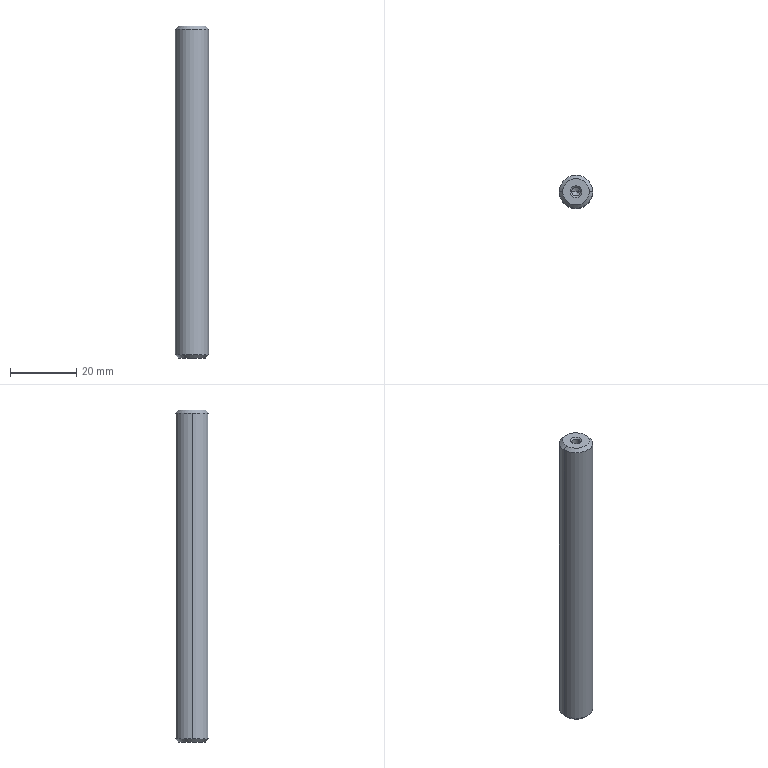Part | SolidWorks | features Chamfer 2, Extrusion 1, HoleWzd 1 | 1 solid | 14 faces | box 10 x 10 x 100 mm | volume 7790 mm3 | cone 8 | cylinder 4 | plane 2 | commonest cylinder face diameters 2.5 x2 10 x2
STEP:
#1=CARTESIAN_POINT('',(-1.25,0.,99.5));
#2=VERTEX_POINT('',#1);
#3=CARTESIAN_POINT('',(1.25,0.,99.5));
#4=VERTEX_POINT('',#3);
#5=CARTESIAN_POINT('',(0.,0.,99.5));
#6=DIRECTION('',(0.,0.,1.));
#7=DIRECTION('',(1.,0.,0.));
#8=AXIS2_PLACEMENT_3D('',#5,#6,#7);
#9=CIRCLE('',#8,1.25);
#10=EDGE_CURVE('',#2,#4,#9,.T.);
#11=ORIENTED_EDGE('',*,*,#10,.F.);
#12=CARTESIAN_POINT('',(-1.75,0.,100.));
#13=VERTEX_POINT('',#12);
#14=CARTESIAN_POINT('',(-1.25,0.,99.5));
#15=DIRECTION('',(-0.7071,0.,0.7071));
#16=VECTOR('',#15,1000.);
#17=LINE('',#14,#16);
#18=EDGE_CURVE('',#2,#13,#17,.T.);
#19=ORIENTED_EDGE('',*,*,#18,.T.);
#20=CARTESIAN_POINT('',(1.75,0.,100.));
#21=VERTEX_POINT('',#20);
#22=CARTESIAN_POINT('',(0.,0.,100.));
#23=DIRECTION('',(0.,0.,-1.));
#24=DIRECTION('',(1.,0.,0.));
#25=AXIS2_PLACEMENT_3D('',#22,#23,#24);
#26=CIRCLE('',#25,1.75);
#27=EDGE_CURVE('',#21,#13,#26,.T.);
#28=ORIENTED_EDGE('',*,*,#27,.F.);
#29=CARTESIAN_POINT('',(1.25,0.,99.5));
#30=DIRECTION('',(0.7071,0.,0.7071));
#31=VECTOR('',#30,1000.);
#32=LINE('',#29,#31);
#33=EDGE_CURVE('',#4,#21,#32,.T.);
#34=ORIENTED_EDGE('',*,*,#33,.F.);
#35=EDGE_LOOP('',(#11,#19,#28,#34));
#36=FACE_OUTER_BOUND('',#35,.T.);
#37=CARTESIAN_POINT('',(0.,0.,99.5));
#38=DIRECTION('',(0.,0.,1.));
#39=DIRECTION('',(1.,0.,0.));
#40=AXIS2_PLACEMENT_3D('',#37,#38,#39);
#41=CONICAL_SURFACE('',#40,1.25,0.7854);
#42=ADVANCED_FACE('',(#36),#41,.F.);
#43=CARTESIAN_POINT('',(4.,0.,100.));
#44=VERTEX_POINT('',#43);
#45=CARTESIAN_POINT('',(-4.,0.,100.));
#46=VERTEX_POINT('',#45);
#47=CARTESIAN_POINT('',(0.,0.,100.));
#48=DIRECTION('',(0.,0.,1.));
#49=DIRECTION('',(1.,0.,0.));
#50=AXIS2_PLACEMENT_3D('',#47,#48,#49);
#51=CIRCLE('',#50,4.);
#52=EDGE_CURVE('',#44,#46,#51,.T.);
#53=ORIENTED_EDGE('',*,*,#52,.F.);
#54=CARTESIAN_POINT('',(5.,0.,99.));
#55=VERTEX_POINT('',#54);
#56=CARTESIAN_POINT('',(4.,0.,100.));
#57=DIRECTION('',(0.7071,0.,-0.7071));
#58=VECTOR('',#57,1000.);
#59=LINE('',#56,#58);
#60=EDGE_CURVE('',#44,#55,#59,.T.);
#61=ORIENTED_EDGE('',*,*,#60,.T.);
#62=CARTESIAN_POINT('',(-5.,0.,99.));
#63=VERTEX_POINT('',#62);
#64=CARTESIAN_POINT('',(0.,0.,99.));
#65=DIRECTION('',(0.,0.,-1.));
#66=DIRECTION('',(1.,0.,0.));
#67=AXIS2_PLACEMENT_3D('',#64,#65,#66);
#68=CIRCLE('',#67,5.);
#69=EDGE_CURVE('',#63,#55,#68,.T.);
#70=ORIENTED_EDGE('',*,*,#69,.F.);
#71=CARTESIAN_POINT('',(-4.,0.,100.));
#72=DIRECTION('',(-0.7071,0.,-0.7071));
#73=VECTOR('',#72,1000.);
#74=LINE('',#71,#73);
#75=EDGE_CURVE('',#46,#63,#74,.T.);
#76=ORIENTED_EDGE('',*,*,#75,.F.);
#77=EDGE_LOOP('',(#53,#61,#70,#76));
#78=FACE_OUTER_BOUND('',#77,.T.);
#79=CARTESIAN_POINT('',(0.,0.,100.));
#80=DIRECTION('',(0.,0.,-1.));
#81=DIRECTION('',(-1.,0.,0.));
#82=AXIS2_PLACEMENT_3D('',#79,#80,#81);
#83=CONICAL_SURFACE('',#82,4.,0.7854);
#84=ADVANCED_FACE('',(#78),#83,.T.);
#85=CARTESIAN_POINT('',(-4.,0.,0.));
#86=VERTEX_POINT('',#85);
#87=CARTESIAN_POINT('',(4.,0.,0.));
#88=VERTEX_POINT('',#87);
#89=CARTESIAN_POINT('',(0.,0.,0.));
#90=DIRECTION('',(0.,0.,-1.));
#91=DIRECTION('',(1.,0.,0.));
#92=AXIS2_PLACEMENT_3D('',#89,#90,#91);
#93=CIRCLE('',#92,4.);
#94=EDGE_CURVE('',#86,#88,#93,.T.);
#95=ORIENTED_EDGE('',*,*,#94,.F.);
#96=CARTESIAN_POINT('',(-5.,0.,1.));
#97=VERTEX_POINT('',#96);
#98=CARTESIAN_POINT('',(-5.,0.,1.));
#99=DIRECTION('',(-0.7071,0.,0.7071));
#100=VECTOR('',#99,1000.);
#101=LINE('',#98,#100);
#102=EDGE_CURVE('',#86,#97,#101,.T.);
#103=ORIENTED_EDGE('',*,*,#102,.T.);
#104=CARTESIAN_POINT('',(5.,0.,1.));
#105=VERTEX_POINT('',#104);
#106=CARTESIAN_POINT('',(0.,0.,1.));
#107=DIRECTION('',(0.,0.,1.));
#108=DIRECTION('',(1.,0.,0.));
#109=AXIS2_PLACEMENT_3D('',#106,#107,#108);
#110=CIRCLE('',#109,5.);
#111=EDGE_CURVE('',#105,#97,#110,.T.);
#112=ORIENTED_EDGE('',*,*,#111,.F.);
#113=CARTESIAN_POINT('',(5.,0.,1.));
#114=DIRECTION('',(0.7071,0.,0.7071));
#115=VECTOR('',#114,1000.);
#116=LINE('',#113,#115);
#117=EDGE_CURVE('',#88,#105,#116,.T.);
#118=ORIENTED_EDGE('',*,*,#117,.F.);
#119=EDGE_LOOP('',(#95,#103,#112,#118));
#120=FACE_OUTER_BOUND('',#119,.T.);
#121=CARTESIAN_POINT('',(0.,0.,1.));
#122=DIRECTION('',(0.,0.,1.));
#123=DIRECTION('',(1.,0.,0.));
#124=AXIS2_PLACEMENT_3D('',#121,#122,#123);
#125=CONICAL_SURFACE('',#124,5.,0.7854);
#126=ADVANCED_FACE('',(#120),#125,.T.);
#127=CARTESIAN_POINT('',(-1.25,0.,93.5));
#128=VERTEX_POINT('',#127);
#129=CARTESIAN_POINT('',(1.25,0.,93.5));
#130=VERTEX_POINT('',#129);
#131=CARTESIAN_POINT('',(0.,0.,93.5));
#132=DIRECTION('',(0.,0.,1.));
#133=DIRECTION('',(1.,0.,0.));
#134=AXIS2_PLACEMENT_3D('',#131,#132,#133);
#135=CIRCLE('',#134,1.25);
#136=EDGE_CURVE('',#128,#130,#135,.T.);
#137=ORIENTED_EDGE('',*,*,#136,.F.);
#138=CARTESIAN_POINT('',(-1.25,0.,100.));
#139=DIRECTION('',(0.,0.,1.));
#140=VECTOR('',#139,1000.);
#141=LINE('',#138,#140);
#142=EDGE_CURVE('',#128,#2,#141,.T.);
#143=ORIENTED_EDGE('',*,*,#142,.T.);
#144=ORIENTED_EDGE('',*,*,#10,.T.);
#145=CARTESIAN_POINT('',(1.25,0.,100.));
#146=DIRECTION('',(0.,0.,1.));
#147=VECTOR('',#146,1000.);
#148=LINE('',#145,#147);
#149=EDGE_CURVE('',#130,#4,#148,.T.);
#150=ORIENTED_EDGE('',*,*,#149,.F.);
#151=EDGE_LOOP('',(#137,#143,#144,#150));
#152=FACE_OUTER_BOUND('',#151,.T.);
#153=CARTESIAN_POINT('',(0.,0.,100.));
#154=DIRECTION('',(0.,0.,1.));
#155=DIRECTION('',(1.,0.,0.));
#156=AXIS2_PLACEMENT_3D('',#153,#154,#155);
#157=CYLINDRICAL_SURFACE('',#156,1.25);
#158=ADVANCED_FACE('',(#152),#157,.F.);
#159=CARTESIAN_POINT('',(0.,0.,92.749));
#160=VERTEX_POINT('',#159);
#161=CARTESIAN_POINT('',(1.25,0.,93.5));
#162=DIRECTION('',(0.8572,0.,0.515));
#163=VECTOR('',#162,1000.);
#164=LINE('',#161,#163);
#165=EDGE_CURVE('',#160,#130,#164,.T.);
#166=ORIENTED_EDGE('',*,*,#165,.F.);
#167=CARTESIAN_POINT('',(-1.25,0.,93.5));
#168=DIRECTION('',(-0.8572,0.,0.515));
#169=VECTOR('',#168,1000.);
#170=LINE('',#167,#169);
#171=EDGE_CURVE('',#160,#128,#170,.T.);
#172=ORIENTED_EDGE('',*,*,#171,.T.);
#173=ORIENTED_EDGE('',*,*,#136,.T.);
#174=EDGE_LOOP('',(#166,#172,#173));
#175=FACE_OUTER_BOUND('',#174,.T.);
#176=CARTESIAN_POINT('',(0.,0.,93.5));
#177=DIRECTION('',(0.,0.,1.));
#178=DIRECTION('',(1.,0.,0.));
#179=AXIS2_PLACEMENT_3D('',#176,#177,#178);
#180=CONICAL_SURFACE('',#179,1.25,1.03);
#181=ADVANCED_FACE('',(#175),#180,.F.);
#182=ORIENTED_EDGE('',*,*,#69,.T.);
#183=CARTESIAN_POINT('',(5.,0.,100.));
#184=DIRECTION('',(0.,0.,-1.));
#185=VECTOR('',#184,1000.);
#186=LINE('',#183,#185);
#187=EDGE_CURVE('',#55,#105,#186,.T.);
#188=ORIENTED_EDGE('',*,*,#187,.T.);
#189=ORIENTED_EDGE('',*,*,#111,.T.);
#190=CARTESIAN_POINT('',(-5.,0.,100.));
#191=DIRECTION('',(0.,0.,-1.));
#192=VECTOR('',#191,1000.);
#193=LINE('',#190,#192);
#194=EDGE_CURVE('',#63,#97,#193,.T.);
#195=ORIENTED_EDGE('',*,*,#194,.F.);
#196=EDGE_LOOP('',(#182,#188,#189,#195));
#197=FACE_OUTER_BOUND('',#196,.T.);
#198=CARTESIAN_POINT('',(0.,0.,100.));
#199=DIRECTION('',(0.,0.,-1.));
#200=DIRECTION('',(-1.,0.,0.));
#201=AXIS2_PLACEMENT_3D('',#198,#199,#200);
#202=CYLINDRICAL_SURFACE('',#201,5.);
#203=ADVANCED_FACE('',(#197),#202,.T.);
#204=ORIENTED_EDGE('',*,*,#187,.F.);
#205=CARTESIAN_POINT('',(0.,0.,99.));
#206=DIRECTION('',(0.,0.,-1.));
#207=DIRECTION('',(1.,0.,0.));
#208=AXIS2_PLACEMENT_3D('',#205,#206,#207);
#209=CIRCLE('',#208,5.);
#210=EDGE_CURVE('',#55,#63,#209,.T.);
#211=ORIENTED_EDGE('',*,*,#210,.T.);
#212=ORIENTED_EDGE('',*,*,#194,.T.);
#213=CARTESIAN_POINT('',(0.,0.,1.));
#214=DIRECTION('',(0.,0.,1.));
#215=DIRECTION('',(1.,0.,0.));
#216=AXIS2_PLACEMENT_3D('',#213,#214,#215);
#217=CIRCLE('',#216,5.);
#218=EDGE_CURVE('',#97,#105,#217,.T.);
#219=ORIENTED_EDGE('',*,*,#218,.T.);
#220=EDGE_LOOP('',(#204,#211,#212,#219));
#221=FACE_OUTER_BOUND('',#220,.T.);
#222=CARTESIAN_POINT('',(0.,0.,100.));
#223=DIRECTION('',(0.,0.,-1.));
#224=DIRECTION('',(-1.,0.,0.));
#225=AXIS2_PLACEMENT_3D('',#222,#223,#224);
#226=CYLINDRICAL_SURFACE('',#225,5.);
#227=ADVANCED_FACE('',(#221),#226,.T.);
#228=ORIENTED_EDGE('',*,*,#27,.T.);
#229=CARTESIAN_POINT('',(0.,0.,100.));
#230=DIRECTION('',(0.,0.,-1.));
#231=DIRECTION('',(1.,0.,0.));
#232=AXIS2_PLACEMENT_3D('',#229,#230,#231);
#233=CIRCLE('',#232,1.75);
#234=EDGE_CURVE('',#13,#21,#233,.T.);
#235=ORIENTED_EDGE('',*,*,#234,.T.);
#236=EDGE_LOOP('',(#228,#235));
#237=FACE_BOUND('',#236,.T.);
#238=CARTESIAN_POINT('',(0.,0.,100.));
#239=DIRECTION('',(0.,0.,1.));
#240=DIRECTION('',(1.,0.,0.));
#241=AXIS2_PLACEMENT_3D('',#238,#239,#240);
#242=CIRCLE('',#241,4.);
#243=EDGE_CURVE('',#46,#44,#242,.T.);
#244=ORIENTED_EDGE('',*,*,#243,.T.);
#245=ORIENTED_EDGE('',*,*,#52,.T.);
#246=EDGE_LOOP('',(#244,#245));
#247=FACE_OUTER_BOUND('',#246,.T.);
#248=CARTESIAN_POINT('',(0.,0.,100.));
#249=DIRECTION('',(0.,0.,1.));
#250=DIRECTION('',(1.,0.,0.));
#251=AXIS2_PLACEMENT_3D('',#248,#249,#250);
#252=PLANE('',#251);
#253=ADVANCED_FACE('',(#237,#247),#252,.T.);
#254=CARTESIAN_POINT('',(0.,0.,0.));
#255=DIRECTION('',(0.,0.,-1.));
#256=DIRECTION('',(1.,0.,0.));
#257=AXIS2_PLACEMENT_3D('',#254,#255,#256);
#258=CIRCLE('',#257,4.);
#259=EDGE_CURVE('',#88,#86,#258,.T.);
#260=ORIENTED_EDGE('',*,*,#259,.T.);
#261=ORIENTED_EDGE('',*,*,#94,.T.);
#262=EDGE_LOOP('',(#260,#261));
#263=FACE_OUTER_BOUND('',#262,.T.);
#264=CARTESIAN_POINT('',(0.,0.,0.));
#265=DIRECTION('',(0.,0.,1.));
#266=DIRECTION('',(1.,0.,0.));
#267=AXIS2_PLACEMENT_3D('',#264,#265,#266);
#268=PLANE('',#267);
#269=ADVANCED_FACE('',(#263),#268,.F.);
#270=ORIENTED_EDGE('',*,*,#171,.F.);
#271=ORIENTED_EDGE('',*,*,#165,.T.);
#272=CARTESIAN_POINT('',(0.,0.,93.5));
#273=DIRECTION('',(0.,0.,1.));
#274=DIRECTION('',(1.,0.,0.));
#275=AXIS2_PLACEMENT_3D('',#272,#273,#274);
#276=CIRCLE('',#275,1.25);
#277=EDGE_CURVE('',#130,#128,#276,.T.);
#278=ORIENTED_EDGE('',*,*,#277,.T.);
#279=EDGE_LOOP('',(#270,#271,#278));
#280=FACE_OUTER_BOUND('',#279,.T.);
#281=CARTESIAN_POINT('',(0.,0.,93.5));
#282=DIRECTION('',(0.,0.,1.));
#283=DIRECTION('',(1.,0.,0.));
#284=AXIS2_PLACEMENT_3D('',#281,#282,#283);
#285=CONICAL_SURFACE('',#284,1.25,1.03);
#286=ADVANCED_FACE('',(#280),#285,.F.);
#287=ORIENTED_EDGE('',*,*,#142,.F.);
#288=ORIENTED_EDGE('',*,*,#277,.F.);
#289=ORIENTED_EDGE('',*,*,#149,.T.);
#290=CARTESIAN_POINT('',(0.,0.,99.5));
#291=DIRECTION('',(0.,0.,1.));
#292=DIRECTION('',(1.,0.,0.));
#293=AXIS2_PLACEMENT_3D('',#290,#291,#292);
#294=CIRCLE('',#293,1.25);
#295=EDGE_CURVE('',#4,#2,#294,.T.);
#296=ORIENTED_EDGE('',*,*,#295,.T.);
#297=EDGE_LOOP('',(#287,#288,#289,#296));
#298=FACE_OUTER_BOUND('',#297,.T.);
#299=CARTESIAN_POINT('',(0.,0.,100.));
#300=DIRECTION('',(0.,0.,1.));
#301=DIRECTION('',(1.,0.,0.));
#302=AXIS2_PLACEMENT_3D('',#299,#300,#301);
#303=CYLINDRICAL_SURFACE('',#302,1.25);
#304=ADVANCED_FACE('',(#298),#303,.F.);
#305=ORIENTED_EDGE('',*,*,#102,.F.);
#306=ORIENTED_EDGE('',*,*,#259,.F.);
#307=ORIENTED_EDGE('',*,*,#117,.T.);
#308=ORIENTED_EDGE('',*,*,#218,.F.);
#309=EDGE_LOOP('',(#305,#306,#307,#308));
#310=FACE_OUTER_BOUND('',#309,.T.);
#311=CARTESIAN_POINT('',(0.,0.,1.));
#312=DIRECTION('',(0.,0.,1.));
#313=DIRECTION('',(1.,0.,0.));
#314=AXIS2_PLACEMENT_3D('',#311,#312,#313);
#315=CONICAL_SURFACE('',#314,5.,0.7854);
#316=ADVANCED_FACE('',(#310),#315,.T.);
#317=ORIENTED_EDGE('',*,*,#60,.F.);
#318=ORIENTED_EDGE('',*,*,#243,.F.);
#319=ORIENTED_EDGE('',*,*,#75,.T.);
#320=ORIENTED_EDGE('',*,*,#210,.F.);
#321=EDGE_LOOP('',(#317,#318,#319,#320));
#322=FACE_OUTER_BOUND('',#321,.T.);
#323=CARTESIAN_POINT('',(0.,0.,100.));
#324=DIRECTION('',(0.,0.,-1.));
#325=DIRECTION('',(-1.,0.,0.));
#326=AXIS2_PLACEMENT_3D('',#323,#324,#325);
#327=CONICAL_SURFACE('',#326,4.,0.7854);
#328=ADVANCED_FACE('',(#322),#327,.T.);
#329=ORIENTED_EDGE('',*,*,#18,.F.);
#330=ORIENTED_EDGE('',*,*,#295,.F.);
#331=ORIENTED_EDGE('',*,*,#33,.T.);
#332=ORIENTED_EDGE('',*,*,#234,.F.);
#333=EDGE_LOOP('',(#329,#330,#331,#332));
#334=FACE_OUTER_BOUND('',#333,.T.);
#335=CARTESIAN_POINT('',(0.,0.,99.5));
#336=DIRECTION('',(0.,0.,1.));
#337=DIRECTION('',(1.,0.,0.));
#338=AXIS2_PLACEMENT_3D('',#335,#336,#337);
#339=CONICAL_SURFACE('',#338,1.25,0.7854);
#340=ADVANCED_FACE('',(#334),#339,.F.);
#341=CLOSED_SHELL('',(#42,#84,#126,#158,#181,#203,#227,#253,#269,#286,#304,#316,#328,#340));
#342=MANIFOLD_SOLID_BREP('',#341);
#343=CARTESIAN_POINT('',(0.,0.,0.));
#344=DIRECTION('',(0.,0.,1.));
#345=DIRECTION('',(1.,0.,0.));
#346=AXIS2_PLACEMENT_3D('',#343,#344,#345);
#347=(LENGTH_UNIT()NAMED_UNIT(*)SI_UNIT(.MILLI.,.METRE.));
#348=UNCERTAINTY_MEASURE_WITH_UNIT(LENGTH_MEASURE(0.00001),#347,'','');
#349=(NAMED_UNIT(*)PLANE_ANGLE_UNIT()SI_UNIT($,.RADIAN.));
#350=(NAMED_UNIT(*)SI_UNIT($,.STERADIAN.)SOLID_ANGLE_UNIT());
#351=(GEOMETRIC_REPRESENTATION_CONTEXT(3)GLOBAL_UNCERTAINTY_ASSIGNED_CONTEXT((#348))GLOBAL_UNIT_ASSIGNED_CONTEXT((#347,#349,#350))REPRESENTATION_CONTEXT('',''));
#352=ADVANCED_BREP_SHAPE_REPRESENTATION('',(#342,#346),#351);